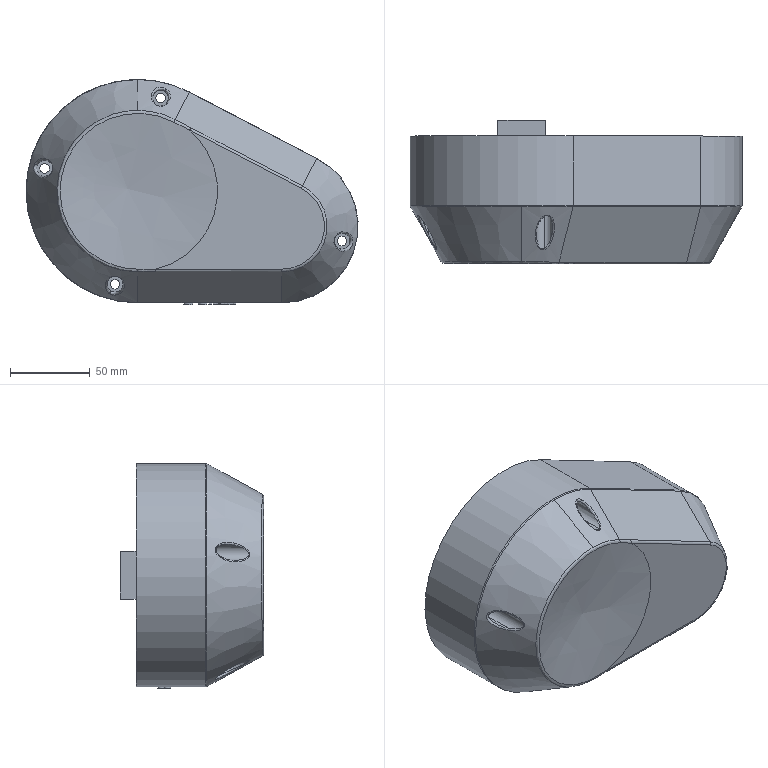Part | SolidWorks | features ICE 3, CirPattern 2, Fillet 2, Chamfer 1, Dome 1, Emboss 1, Extrusion 1, PLine 1 | 1 solid | 129 faces | box 208 x 90 x 141 mm | volume 1602539 mm3 | spline 58 | plane 43 | cylinder 22 | torus 3 | cone 3 | commonest cylinder face diameters 6 x8 10 x8 4 x4 96 x1 140 x1